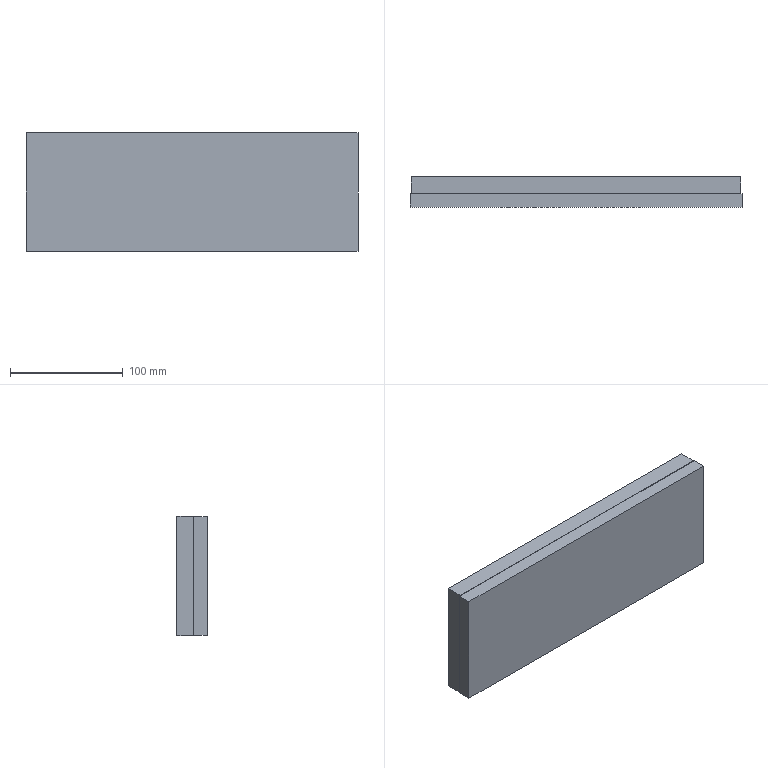NC program | NX | posted with a generic post | part box 295 x 27 x 106 mm
Lines 3310 to 4614 of 7486:
(PLANAR_MILL_6 , TOOL : D4R0)
N6474 T06 M6
N6476 G54
N6478 G17 G0 G90 X25.171 Y86.748 S3000 M3
N6480 G43 Z20. H6
N6482 Z0.3
N6484 G94 G1 X25.263 Y86.696 Z0.296 F400.
N6486 X25.737 Z0.28
N6488 X26.172 Y86.944 Z0.262
N6490 X26.42 Y87.379 Z0.245
N6492 Y87.852 Z0.228
N6494 X26.172 Y88.287 Z0.211
N6496 X25.737 Y88.536 Z0.193
N6498 X25.263 Z0.177
N6500 X24.828 Y88.287 Z0.159
N6502 X24.58 Y87.852 Z0.142
N6504 Y87.379 Z0.125
N6506 X24.828 Y86.944 Z0.108
N6508 X25.263 Y86.696 Z0.09
N6510 X25.737 Z0.074
N6512 X26.172 Y86.944 Z0.056
N6514 X26.42 Y87.379 Z0.039
N6516 Y87.852 Z0.022
N6518 X26.172 Y88.287 Z0.005
N6520 X25.737 Y88.536 Z-0.013
N6522 X25.263 Z-0.029
N6524 X24.828 Y88.287 Z-0.047
N6526 X24.58 Y87.852 Z-0.064
N6528 Y87.379 Z-0.081
N6530 X24.828 Y86.944 Z-0.098
N6532 X25.263 Y86.696 Z-0.116
N6534 X25.737 Z-0.132
N6536 X26.172 Y86.944 Z-0.15
N6538 X26.42 Y87.379 Z-0.167
N6540 Y87.852 Z-0.184
N6542 X26.172 Y88.287 Z-0.201
N6544 X25.737 Y88.536 Z-0.219
N6546 X25.263 Z-0.235
N6548 X24.828 Y88.287 Z-0.253
N6550 X24.58 Y87.852 Z-0.27
N6552 Y87.379 Z-0.287
N6554 X24.828 Y86.944 Z-0.304
N6556 X25.263 Y86.696 Z-0.322
N6558 X25.737 Z-0.338
N6560 X26.172 Y86.944 Z-0.356
N6562 X26.42 Y87.379 Z-0.373
N6564 Y87.852 Z-0.39
N6566 X26.172 Y88.287 Z-0.407
N6568 X25.737 Y88.536 Z-0.425
N6570 X25.263 Z-0.441
N6572 X24.828 Y88.287 Z-0.459
N6574 X24.58 Y87.852 Z-0.476
N6576 Y87.379 Z-0.493
N6578 X24.828 Y86.944 Z-0.51
N6580 X25.263 Y86.696 Z-0.528
N6582 X25.737 Z-0.545
N6584 X26.172 Y86.944 Z-0.562
N6586 X26.42 Y87.379 Z-0.579
N6588 Y87.852 Z-0.596
N6590 X26.172 Y88.287 Z-0.614
N6592 X25.737 Y88.536 Z-0.631
N6594 X25.263 Z-0.648
N6596 X24.828 Y88.287 Z-0.665
N6598 X24.58 Y87.852 Z-0.683
N6600 Y87.379 Z-0.699
N6602 X24.828 Y86.944 Z-0.717
N6604 X25.263 Y86.696 Z-0.734
N6606 X25.737 Z-0.751
N6608 X26.172 Y86.944 Z-0.768
N6610 X26.42 Y87.379 Z-0.786
N6612 Y87.852 Z-0.802
N6614 X26.172 Y88.287 Z-0.82
N6616 X25.737 Y88.536 Z-0.837
N6618 X25.263 Z-0.854
N6620 X24.828 Y88.287 Z-0.871
N6622 X24.58 Y87.852 Z-0.889
N6624 Y87.379 Z-0.905
N6626 X24.828 Y86.944 Z-0.923
N6628 X25.263 Y86.696 Z-0.94
N6630 X25.737 Z-0.957
N6632 X26.172 Y86.944 Z-0.974
N6634 X26.42 Y87.379 Z-0.992
N6636 Y87.852 Z-1.008
N6638 X26.172 Y88.287 Z-1.026
N6640 X25.737 Y88.536 Z-1.043
N6642 X25.263 Z-1.06
N6644 X24.828 Y88.287 Z-1.077
N6646 X24.58 Y87.852 Z-1.095
N6648 Y87.379 Z-1.111
N6650 X24.828 Y86.944 Z-1.129
N6652 X25.263 Y86.696 Z-1.146
N6654 X25.737 Z-1.163
N6656 X26.172 Y86.944 Z-1.18
N6658 X26.42 Y87.379 Z-1.198
N6660 Y87.852 Z-1.214
N6662 X26.172 Y88.287 Z-1.232
N6664 X25.737 Y88.536 Z-1.249
N6666 X25.263 Z-1.266
N6668 X24.828 Y88.287 Z-1.283
N6670 X24.58 Y87.852 Z-1.301
N6672 Y87.379 Z-1.317
N6674 X24.828 Y86.944 Z-1.335
N6676 X25.263 Y86.696 Z-1.352
N6678 X25.737 Z-1.369
N6680 X26.172 Y86.944 Z-1.386
N6682 X26.42 Y87.379 Z-1.404
N6684 Y87.852 Z-1.42
N6686 X26.172 Y88.287 Z-1.438
N6688 X25.737 Y88.536 Z-1.455
N6690 X25.263 Z-1.472
N6692 X24.828 Y88.287 Z-1.489
N6694 X24.58 Y87.852 Z-1.507
N6696 Y87.379 Z-1.523
N6698 X24.828 Y86.944 Z-1.541
N6700 X25.263 Y86.696 Z-1.558
N6702 X25.737 Z-1.575
N6704 X26.172 Y86.944 Z-1.592
N6706 X26.42 Y87.379 Z-1.61
N6708 Y87.852 Z-1.626
N6710 X26.172 Y88.287 Z-1.644
N6712 X25.737 Y88.536 Z-1.661
N6714 X25.263 Z-1.678
N6716 X24.828 Y88.287 Z-1.695
N6718 X24.58 Y87.852 Z-1.713
N6720 Y87.379 Z-1.729
N6722 X24.828 Y86.944 Z-1.747
N6724 X25.263 Y86.696 Z-1.764
N6726 X25.737 Z-1.781
N6728 X26.172 Y86.944 Z-1.798
N6730 X26.42 Y87.379 Z-1.816
N6732 Y87.852 Z-1.832
N6734 X26.172 Y88.287 Z-1.85
N6736 X25.737 Y88.536 Z-1.867
N6738 X25.263 Z-1.884
N6740 X24.828 Y88.287 Z-1.901
N6742 X24.58 Y87.852 Z-1.919
N6744 Y87.379 Z-1.935
N6746 X24.828 Y86.944 Z-1.953
N6748 X25.263 Y86.696 Z-1.97
N6750 X25.737 Z-1.987
N6752 X26.172 Y86.944 Z-2.004
N6754 X26.42 Y87.379 Z-2.022
N6756 Y87.852 Z-2.038
N6758 X26.172 Y88.287 Z-2.056
N6760 X25.737 Y88.536 Z-2.073
N6762 X25.263 Z-2.09
N6764 X24.828 Y88.287 Z-2.107
N6766 X24.58 Y87.852 Z-2.125
N6768 Y87.379 Z-2.142
N6770 X24.828 Y86.944 Z-2.159
N6772 X25.263 Y86.696 Z-2.176
N6774 X25.737 Z-2.193
N6776 X26.172 Y86.944 Z-2.211
N6778 X26.42 Y87.379 Z-2.228
N6780 Y87.852 Z-2.245
N6782 X26.172 Y88.287 Z-2.262
N6784 X25.737 Y88.536 Z-2.28
N6786 X25.263 Z-2.296
N6788 X24.828 Y88.287 Z-2.314
N6790 X24.58 Y87.852 Z-2.331
N6792 Y87.379 Z-2.348
N6794 X24.828 Y86.944 Z-2.365
N6796 X25.263 Y86.696 Z-2.383
N6798 X25.737 Z-2.399
N6800 X26.172 Y86.944 Z-2.417
N6802 X26.42 Y87.379 Z-2.434
N6804 Y87.852 Z-2.451
N6806 X26.172 Y88.287 Z-2.468
N6808 X25.737 Y88.536 Z-2.486
N6810 X25.263 Z-2.502
N6812 X24.828 Y88.287 Z-2.52
N6814 X24.58 Y87.852 Z-2.537
N6816 Y87.379 Z-2.554
N6818 X24.828 Y86.944 Z-2.571
N6820 X25.263 Y86.696 Z-2.589
N6822 X25.737 Z-2.605
N6824 X26.172 Y86.944 Z-2.623
N6826 X26.42 Y87.379 Z-2.64
N6828 Y87.852 Z-2.657
N6830 X26.172 Y88.287 Z-2.674
N6832 X25.737 Y88.536 Z-2.692
N6834 X25.263 Z-2.708
N6836 X24.828 Y88.287 Z-2.726
N6838 X24.58 Y87.852 Z-2.743
N6840 Y87.379 Z-2.76
N6842 X24.828 Y86.944 Z-2.777
N6844 X25.263 Y86.696 Z-2.795
N6846 X25.737 Z-2.811
N6848 X26.172 Y86.944 Z-2.829
N6850 X26.42 Y87.379 Z-2.846
N6852 Y87.852 Z-2.863
N6854 X26.172 Y88.287 Z-2.88
N6856 X25.737 Y88.536 Z-2.898
N6858 X25.263 Z-2.914
N6860 X24.828 Y88.287 Z-2.932
N6862 X24.58 Y87.852 Z-2.949
N6864 Y87.379 Z-2.966
N6866 X24.828 Y86.944 Z-2.983
N6868 X25.263 Y86.696 Z-3.001
N6870 X25.737 Z-3.017
N6872 X26.172 Y86.944 Z-3.035
N6874 X26.42 Y87.379 Z-3.052
N6876 Y87.852 Z-3.069
N6878 X26.172 Y88.287 Z-3.086
N6880 X25.737 Y88.536 Z-3.104
N6882 X25.263 Z-3.12
N6884 X24.828 Y88.287 Z-3.138
N6886 X24.58 Y87.852 Z-3.155
N6888 Y87.379 Z-3.172
N6890 X24.828 Y86.944 Z-3.189
N6892 X25.263 Y86.696 Z-3.207
N6894 X25.737 Z-3.223
N6896 X26.172 Y86.944 Z-3.241
N6898 X26.42 Y87.379 Z-3.258
N6900 Y87.852 Z-3.275
N6902 X26.172 Y88.287 Z-3.292
N6904 X25.737 Y88.536 Z-3.31
N6906 X25.263 Z-3.326
N6908 X24.828 Y88.287 Z-3.344
N6910 X24.58 Y87.852 Z-3.361
N6912 Y87.379 Z-3.378
N6914 X24.828 Y86.944 Z-3.395
N6916 X25.263 Y86.696 Z-3.413
N6918 X25.737 Z-3.429
N6920 X26.172 Y86.944 Z-3.447
N6922 X26.42 Y87.379 Z-3.464
N6924 Y87.852 Z-3.481
N6926 X26.172 Y88.287 Z-3.498
N6928 X25.737 Y88.536 Z-3.516
N6930 X25.263 Z-3.532
N6932 X24.828 Y88.287 Z-3.55
N6934 X24.58 Y87.852 Z-3.567
N6936 Y87.379 Z-3.584
N6938 X24.828 Y86.944 Z-3.601
N6940 X25.263 Y86.696 Z-3.619
N6942 X25.737 Z-3.635
N6944 X26.172 Y86.944 Z-3.653
N6946 X26.42 Y87.379 Z-3.67
N6948 Y87.852 Z-3.687
N6950 X26.172 Y88.287 Z-3.704
N6952 X25.737 Y88.536 Z-3.722
N6954 X25.263 Z-3.739
N6956 X24.828 Y88.287 Z-3.756
N6958 X24.58 Y87.852 Z-3.773
N6960 Y87.379 Z-3.79
N6962 X24.828 Y86.944 Z-3.808
N6964 X25.263 Y86.696 Z-3.825
N6966 X25.737 Z-3.842
N6968 X26.172 Y86.944 Z-3.859
N6970 X26.42 Y87.379 Z-3.877
N6972 Y87.852 Z-3.893
N6974 X26.172 Y88.287 Z-3.911
N6976 X25.737 Y88.536 Z-3.928
N6978 X25.263 Z-3.945
N6980 X24.828 Y88.287 Z-3.962
N6982 X24.58 Y87.852 Z-3.98
N6984 Y87.379 Z-3.996
N6986 X24.828 Y86.944 Z-4.014
N6988 X25.263 Y86.696 Z-4.031
N6990 X25.737 Z-4.048
N6992 X26.172 Y86.944 Z-4.065
N6994 X26.42 Y87.379 Z-4.083
N6996 Y87.852 Z-4.099
N6998 X26.172 Y88.287 Z-4.117
N7000 X25.737 Y88.536 Z-4.134
N7002 X25.263 Z-4.151
N7004 X24.828 Y88.287 Z-4.168
N7006 X24.58 Y87.852 Z-4.186
N7008 Y87.379 Z-4.202
N7010 X24.828 Y86.944 Z-4.22
N7012 X25.263 Y86.696 Z-4.237
N7014 X25.737 Z-4.254
N7016 X26.172 Y86.944 Z-4.271
N7018 X26.42 Y87.379 Z-4.289
N7020 Y87.852 Z-4.305
N7022 X26.172 Y88.287 Z-4.323
N7024 X25.737 Y88.536 Z-4.34
N7026 X25.263 Z-4.357
N7028 X24.828 Y88.287 Z-4.374
N7030 X24.58 Y87.852 Z-4.392
N7032 Y87.379 Z-4.408
N7034 X24.828 Y86.944 Z-4.426
N7036 X25.263 Y86.696 Z-4.443
N7038 X25.737 Z-4.46
N7040 X26.172 Y86.944 Z-4.477
N7042 X26.42 Y87.379 Z-4.495
N7044 Y87.852 Z-4.511
N7046 X26.172 Y88.287 Z-4.529
N7048 X25.737 Y88.536 Z-4.546
N7050 X25.263 Z-4.563
N7052 X24.828 Y88.287 Z-4.58
N7054 X24.58 Y87.852 Z-4.598
N7056 Y87.379 Z-4.614
N7058 X24.828 Y86.944 Z-4.632
N7060 X25.263 Y86.696 Z-4.649
N7062 X25.737 Z-4.666
N7064 X26.172 Y86.944 Z-4.683
N7066 X26.42 Y87.379 Z-4.701
N7068 Y87.852 Z-4.717
N7070 X26.172 Y88.287 Z-4.735
N7072 X25.737 Y88.536 Z-4.752
N7074 X25.263 Z-4.769
N7076 X24.828 Y88.287 Z-4.786
N7078 X24.58 Y87.852 Z-4.804
N7080 Y87.379 Z-4.82
N7082 X24.828 Y86.944 Z-4.838
N7084 X25.263 Y86.696 Z-4.855
N7086 X25.737 Z-4.872
N7088 X26.172 Y86.944 Z-4.889
N7090 X26.42 Y87.379 Z-4.907
N7092 Y87.852 Z-4.923
N7094 X26.172 Y88.287 Z-4.941
N7096 X25.737 Y88.536 Z-4.958
N7098 X25.263 Z-4.975
N7100 X24.828 Y88.287 Z-4.992
N7102 X24.58 Y87.852 Z-5.01
N7104 Y87.379 Z-5.026
N7106 X24.828 Y86.944 Z-5.044
N7108 X25.263 Y86.696 Z-5.061
N7110 X25.737 Z-5.078
N7112 X26.172 Y86.944 Z-5.095
N7114 X26.42 Y87.379 Z-5.113
N7116 Y87.852 Z-5.129
N7118 X26.172 Y88.287 Z-5.147
N7120 X25.737 Y88.536 Z-5.164
N7122 X25.263 Z-5.181
N7124 X24.828 Y88.287 Z-5.198
N7126 X24.58 Y87.852 Z-5.216
N7128 Y87.379 Z-5.232
N7130 X24.828 Y86.944 Z-5.25
N7132 X25.263 Y86.696 Z-5.267
N7134 X25.737 Z-5.284
N7136 X26.172 Y86.944 Z-5.301
N7138 X26.42 Y87.379 Z-5.319
N7140 Y87.852 Z-5.336
N7142 X26.172 Y88.287 Z-5.353
N7144 X25.737 Y88.536 Z-5.371
N7146 X25.263 Z-5.387
N7148 X24.828 Y88.287 Z-5.405
N7150 X24.58 Y87.852 Z-5.422
N7152 Y87.379 Z-5.439
N7154 X24.828 Y86.944 Z-5.456
N7156 X25.263 Y86.696 Z-5.474
N7158 X25.737 Z-5.49
N7160 X26.172 Y86.944 Z-5.508
N7162 X26.42 Y87.379 Z-5.525
N7164 Y87.852 Z-5.542
N7166 X26.172 Y88.287 Z-5.559
N7168 X25.737 Y88.536 Z-5.577
N7170 X25.263 Z-5.593
N7172 X24.828 Y88.287 Z-5.611
N7174 X24.58 Y87.852 Z-5.628
N7176 Y87.379 Z-5.645
N7178 X24.828 Y86.944 Z-5.662
N7180 X25.263 Y86.696 Z-5.68
N7182 X25.737 Z-5.696
N7184 X26.172 Y86.944 Z-5.714
N7186 X26.42 Y87.379 Z-5.731
N7188 Y87.852 Z-5.748
N7190 X26.172 Y88.287 Z-5.765
N7192 X25.737 Y88.536 Z-5.783
N7194 X25.263 Z-5.799
N7196 X24.828 Y88.287 Z-5.817
N7198 X24.58 Y87.852 Z-5.834
N7200 Y87.379 Z-5.851
N7202 X24.828 Y86.944 Z-5.868
N7204 X25.263 Y86.696 Z-5.886
N7206 X25.737 Z-5.902
N7208 X26.172 Y86.944 Z-5.92
N7210 X26.42 Y87.379 Z-5.937
N7212 Y87.852 Z-5.954
N7214 X26.172 Y88.287 Z-5.971
N7216 X25.737 Y88.536 Z-5.989
N7218 X25.263 Z-6.005
N7220 X24.828 Y88.287 Z-6.023
N7222 X24.58 Y87.852 Z-6.04
N7224 Y87.379 Z-6.057
N7226 X24.828 Y86.944 Z-6.074
N7228 X25.263 Y86.696 Z-6.092
N7230 X25.5 Z-6.1
N7232 G3 X26.42 Y87.616 R0.92
N7234 X25.5 Y86.696 R-0.92
N7236 G1 Z-5.8
N7238 G0 Z20.
N7240 X244.171 Y48.133
N7242 Z0.3
N7244 G1 X244.263 Y48.08 Z0.296
N7246 X244.737 Z0.28
N7248 X245.172 Y48.328 Z0.262
N7250 X245.42 Y48.763 Z0.245
N7252 Y49.237 Z0.228
N7254 X245.172 Y49.672 Z0.211
N7256 X244.737 Y49.92 Z0.193
N7258 X244.263 Z0.177
N7260 X243.828 Y49.672 Z0.159
N7262 X243.58 Y49.237 Z0.142
N7264 Y48.763 Z0.125
N7266 X243.828 Y48.328 Z0.108
N7268 X244.263 Y48.08 Z0.09
N7270 X244.737 Z0.074
N7272 X245.172 Y48.328 Z0.056
N7274 X245.42 Y48.763 Z0.039
N7276 Y49.237 Z0.022
N7278 X245.172 Y49.672 Z0.005
N7280 X244.737 Y49.92 Z-0.013
N7282 X244.263 Z-0.029
N7284 X243.828 Y49.672 Z-0.047
N7286 X243.58 Y49.237 Z-0.064
N7288 Y48.763 Z-0.081
N7290 X243.828 Y48.328 Z-0.098
N7292 X244.263 Y48.08 Z-0.116
N7294 X244.737 Z-0.132
N7296 X245.172 Y48.328 Z-0.15
N7298 X245.42 Y48.763 Z-0.167
N7300 Y49.237 Z-0.184
N7302 X245.172 Y49.672 Z-0.201
N7304 X244.737 Y49.92 Z-0.219
N7306 X244.263 Z-0.235
N7308 X243.828 Y49.672 Z-0.253
N7310 X243.58 Y49.237 Z-0.27
N7312 Y48.763 Z-0.287
N7314 X243.828 Y48.328 Z-0.304
N7316 X244.263 Y48.08 Z-0.322
N7318 X244.737 Z-0.338
N7320 X245.172 Y48.328 Z-0.356
N7322 X245.42 Y48.763 Z-0.373
N7324 Y49.237 Z-0.39
N7326 X245.172 Y49.672 Z-0.407
N7328 X244.737 Y49.92 Z-0.425
N7330 X244.263 Z-0.441
N7332 X243.828 Y49.672 Z-0.459
N7334 X243.58 Y49.237 Z-0.476
N7336 Y48.763 Z-0.493
N7338 X243.828 Y48.328 Z-0.51
N7340 X244.263 Y48.08 Z-0.528
N7342 X244.737 Z-0.545
N7344 X245.172 Y48.328 Z-0.562
N7346 X245.42 Y48.763 Z-0.579
N7348 Y49.237 Z-0.596
N7350 X245.172 Y49.672 Z-0.614
N7352 X244.737 Y49.92 Z-0.631
N7354 X244.263 Z-0.648
N7356 X243.828 Y49.672 Z-0.665
N7358 X243.58 Y49.237 Z-0.683
N7360 Y48.763 Z-0.699
N7362 X243.828 Y48.328 Z-0.717
N7364 X244.263 Y48.08 Z-0.734
N7366 X244.737 Z-0.751
N7368 X245.172 Y48.328 Z-0.768
N7370 X245.42 Y48.763 Z-0.786
N7372 Y49.237 Z-0.802
N7374 X245.172 Y49.672 Z-0.82
N7376 X244.737 Y49.92 Z-0.837
N7378 X244.263 Z-0.854
N7380 X243.828 Y49.672 Z-0.871
N7382 X243.58 Y49.237 Z-0.889
N7384 Y48.763 Z-0.905
N7386 X243.828 Y48.328 Z-0.923
N7388 X244.263 Y48.08 Z-0.94
N7390 X244.737 Z-0.957
N7392 X245.172 Y48.328 Z-0.974
N7394 X245.42 Y48.763 Z-0.992
N7396 Y49.237 Z-1.008
N7398 X245.172 Y49.672 Z-1.026
N7400 X244.737 Y49.92 Z-1.043
N7402 X244.263 Z-1.06
N7404 X243.828 Y49.672 Z-1.077
N7406 X243.58 Y49.237 Z-1.095
N7408 Y48.763 Z-1.111
N7410 X243.828 Y48.328 Z-1.129
N7412 X244.263 Y48.08 Z-1.146
N7414 X244.737 Z-1.163
N7416 X245.172 Y48.328 Z-1.18
N7418 X245.42 Y48.763 Z-1.198
N7420 Y49.237 Z-1.214
N7422 X245.172 Y49.672 Z-1.232
N7424 X244.737 Y49.92 Z-1.249
N7426 X244.263 Z-1.266
N7428 X243.828 Y49.672 Z-1.283
N7430 X243.58 Y49.237 Z-1.301
N7432 Y48.763 Z-1.317
N7434 X243.828 Y48.328 Z-1.335
N7436 X244.263 Y48.08 Z-1.352
N7438 X244.737 Z-1.369
N7440 X245.172 Y48.328 Z-1.386
N7442 X245.42 Y48.763 Z-1.404
N7444 Y49.237 Z-1.42
N7446 X245.172 Y49.672 Z-1.438
N7448 X244.737 Y49.92 Z-1.455
N7450 X244.263 Z-1.472
N7452 X243.828 Y49.672 Z-1.489
N7454 X243.58 Y49.237 Z-1.507
N7456 Y48.763 Z-1.523
N7458 X243.828 Y48.328 Z-1.541
N7460 X244.263 Y48.08 Z-1.558
N7462 X244.737 Z-1.575
N7464 X245.172 Y48.328 Z-1.592
N7466 X245.42 Y48.763 Z-1.61
N7468 Y49.237 Z-1.626
N7470 X245.172 Y49.672 Z-1.644
N7472 X244.737 Y49.92 Z-1.661
N7474 X244.263 Z-1.678
N7476 X243.828 Y49.672 Z-1.695
N7478 X243.58 Y49.237 Z-1.713
N7480 Y48.763 Z-1.729
N7482 X243.828 Y48.328 Z-1.747
N7484 X244.263 Y48.08 Z-1.764
N7486 X244.737 Z-1.781
N7488 X245.172 Y48.328 Z-1.798
N7490 X245.42 Y48.763 Z-1.816
N7492 Y49.237 Z-1.832
N7494 X245.172 Y49.672 Z-1.85
N7496 X244.737 Y49.92 Z-1.867
N7498 X244.263 Z-1.884
N7500 X243.828 Y49.672 Z-1.901
N7502 X243.58 Y49.237 Z-1.919
N7504 Y48.763 Z-1.935
N7506 X243.828 Y48.328 Z-1.953
N7508 X244.263 Y48.08 Z-1.97
N7510 X244.737 Z-1.987
N7512 X245.172 Y48.328 Z-2.004
N7514 X245.42 Y48.763 Z-2.022
N7516 Y49.237 Z-2.038
N7518 X245.172 Y49.672 Z-2.056
N7520 X244.737 Y49.92 Z-2.073
N7522 X244.263 Z-2.09
N7524 X243.828 Y49.672 Z-2.107
N7526 X243.58 Y49.237 Z-2.125
N7528 Y48.763 Z-2.142
N7530 X243.828 Y48.328 Z-2.159
N7532 X244.263 Y48.08 Z-2.176
N7534 X244.737 Z-2.193
N7536 X245.172 Y48.328 Z-2.211
N7538 X245.42 Y48.763 Z-2.228
N7540 Y49.237 Z-2.245
N7542 X245.172 Y49.672 Z-2.262
N7544 X244.737 Y49.92 Z-2.28
N7546 X244.263 Z-2.296
N7548 X243.828 Y49.672 Z-2.314
N7550 X243.58 Y49.237 Z-2.331
N7552 Y48.763 Z-2.348
N7554 X243.828 Y48.328 Z-2.365
N7556 X244.263 Y48.08 Z-2.383
N7558 X244.737 Z-2.399
N7560 X245.172 Y48.328 Z-2.417
N7562 X245.42 Y48.763 Z-2.434
N7564 Y49.237 Z-2.451
N7566 X245.172 Y49.672 Z-2.468
N7568 X244.737 Y49.92 Z-2.486
N7570 X244.263 Z-2.502
N7572 X243.828 Y49.672 Z-2.52
N7574 X243.58 Y49.237 Z-2.537
N7576 Y48.763 Z-2.554
N7578 X243.828 Y48.328 Z-2.571
N7580 X244.263 Y48.08 Z-2.589
N7582 X244.737 Z-2.605
N7584 X245.172 Y48.328 Z-2.623
N7586 X245.42 Y48.763 Z-2.64
N7588 Y49.237 Z-2.657
N7590 X245.172 Y49.672 Z-2.674
N7592 X244.737 Y49.92 Z-2.692
N7594 X244.263 Z-2.708
N7596 X243.828 Y49.672 Z-2.726
N7598 X243.58 Y49.237 Z-2.743
N7600 Y48.763 Z-2.76
N7602 X243.828 Y48.328 Z-2.777
N7604 X244.263 Y48.08 Z-2.795
N7606 X244.737 Z-2.811
N7608 X245.172 Y48.328 Z-2.829
N7610 X245.42 Y48.763 Z-2.846
N7612 Y49.237 Z-2.863
N7614 X245.172 Y49.672 Z-2.88
N7616 X244.737 Y49.92 Z-2.898
N7618 X244.263 Z-2.914
N7620 X243.828 Y49.672 Z-2.932
N7622 X243.58 Y49.237 Z-2.949
N7624 Y48.763 Z-2.966
N7626 X243.828 Y48.328 Z-2.983
N7628 X244.263 Y48.08 Z-3.001
N7630 X244.737 Z-3.017
N7632 X245.172 Y48.328 Z-3.035
N7634 X245.42 Y48.763 Z-3.052
N7636 Y49.237 Z-3.069
N7638 X245.172 Y49.672 Z-3.086
N7640 X244.737 Y49.92 Z-3.104
N7642 X244.263 Z-3.12
N7644 X243.828 Y49.672 Z-3.138
N7646 X243.58 Y49.237 Z-3.155
N7648 Y48.763 Z-3.172
N7650 X243.828 Y48.328 Z-3.189
N7652 X244.263 Y48.08 Z-3.207
N7654 X244.737 Z-3.223
N7656 X245.172 Y48.328 Z-3.241
N7658 X245.42 Y48.763 Z-3.258
N7660 Y49.237 Z-3.275
N7662 X245.172 Y49.672 Z-3.292
N7664 X244.737 Y49.92 Z-3.31
N7666 X244.263 Z-3.326
N7668 X243.828 Y49.672 Z-3.344
N7670 X243.58 Y49.237 Z-3.361
N7672 Y48.763 Z-3.378
N7674 X243.828 Y48.328 Z-3.395
N7676 X244.263 Y48.08 Z-3.413
N7678 X244.737 Z-3.429
N7680 X245.172 Y48.328 Z-3.447
N7682 X245.42 Y48.763 Z-3.464
N7684 Y49.237 Z-3.481
N7686 X245.172 Y49.672 Z-3.498
N7688 X244.737 Y49.92 Z-3.516
N7690 X244.263 Z-3.532
N7692 X243.828 Y49.672 Z-3.55
N7694 X243.58 Y49.237 Z-3.567
N7696 Y48.763 Z-3.584
N7698 X243.828 Y48.328 Z-3.601
N7700 X244.263 Y48.08 Z-3.619
N7702 X244.737 Z-3.635
N7704 X245.172 Y48.328 Z-3.653
N7706 X245.42 Y48.763 Z-3.67
N7708 Y49.237 Z-3.687
N7710 X245.172 Y49.672 Z-3.704
N7712 X244.737 Y49.92 Z-3.722
N7714 X244.263 Z-3.739
N7716 X243.828 Y49.672 Z-3.756
N7718 X243.58 Y49.237 Z-3.773
N7720 Y48.763 Z-3.79
N7722 X243.828 Y48.328 Z-3.808
N7724 X244.263 Y48.08 Z-3.825
N7726 X244.737 Z-3.842
N7728 X245.172 Y48.328 Z-3.859
N7730 X245.42 Y48.763 Z-3.877
N7732 Y49.237 Z-3.893
N7734 X245.172 Y49.672 Z-3.911
N7736 X244.737 Y49.92 Z-3.928
N7738 X244.263 Z-3.945
N7740 X243.828 Y49.672 Z-3.962
N7742 X243.58 Y49.237 Z-3.98
N7744 Y48.763 Z-3.996
N7746 X243.828 Y48.328 Z-4.014
N7748 X244.263 Y48.08 Z-4.031
N7750 X244.737 Z-4.048
N7752 X245.172 Y48.328 Z-4.065
N7754 X245.42 Y48.763 Z-4.083
N7756 Y49.237 Z-4.099
N7758 X245.172 Y49.672 Z-4.117
N7760 X244.737 Y49.92 Z-4.134
N7762 X244.263 Z-4.151
N7764 X243.828 Y49.672 Z-4.168
N7766 X243.58 Y49.237 Z-4.186
N7768 Y48.763 Z-4.202
N7770 X243.828 Y48.328 Z-4.22
N7772 X244.263 Y48.08 Z-4.237
N7774 X244.737 Z-4.254
N7776 X245.172 Y48.328 Z-4.271
N7778 X245.42 Y48.763 Z-4.289
N7780 Y49.237 Z-4.305
N7782 X245.172 Y49.672 Z-4.323
N7784 X244.737 Y49.92 Z-4.34
N7786 X244.263 Z-4.357
N7788 X243.828 Y49.672 Z-4.374
N7790 X243.58 Y49.237 Z-4.392
N7792 Y48.763 Z-4.408
N7794 X243.828 Y48.328 Z-4.426
N7796 X244.263 Y48.08 Z-4.443
N7798 X244.737 Z-4.46
N7800 X245.172 Y48.328 Z-4.477
N7802 X245.42 Y48.763 Z-4.495
N7804 Y49.237 Z-4.511
N7806 X245.172 Y49.672 Z-4.529
N7808 X244.737 Y49.92 Z-4.546
N7810 X244.263 Z-4.563
N7812 X243.828 Y49.672 Z-4.58
N7814 X243.58 Y49.237 Z-4.598
N7816 Y48.763 Z-4.614
N7818 X243.828 Y48.328 Z-4.632
N7820 X244.263 Y48.08 Z-4.649
N7822 X244.737 Z-4.666
N7824 X245.172 Y48.328 Z-4.683
N7826 X245.42 Y48.763 Z-4.701
N7828 Y49.237 Z-4.717
N7830 X245.172 Y49.672 Z-4.735
N7832 X244.737 Y49.92 Z-4.752
N7834 X244.263 Z-4.769
N7836 X243.828 Y49.672 Z-4.786
N7838 X243.58 Y49.237 Z-4.804
N7840 Y48.763 Z-4.82
N7842 X243.828 Y48.328 Z-4.838
N7844 X244.263 Y48.08 Z-4.855
N7846 X244.737 Z-4.872
N7848 X245.172 Y48.328 Z-4.889
N7850 X245.42 Y48.763 Z-4.907
N7852 Y49.237 Z-4.923
N7854 X245.172 Y49.672 Z-4.941
N7856 X244.737 Y49.92 Z-4.958
N7858 X244.263 Z-4.975
N7860 X243.828 Y49.672 Z-4.992
N7862 X243.58 Y49.237 Z-5.01
N7864 Y48.763 Z-5.026
N7866 X243.828 Y48.328 Z-5.044
N7868 X244.263 Y48.08 Z-5.061
N7870 X244.737 Z-5.078
N7872 X245.172 Y48.328 Z-5.095
N7874 X245.42 Y48.763 Z-5.113
N7876 Y49.237 Z-5.129
N7878 X245.172 Y49.672 Z-5.147
N7880 X244.737 Y49.92 Z-5.164
N7882 X244.263 Z-5.181
N7884 X243.828 Y49.672 Z-5.198
N7886 X243.58 Y49.237 Z-5.216
N7888 Y48.763 Z-5.232
N7890 X243.828 Y48.328 Z-5.25
N7892 X244.263 Y48.08 Z-5.267
N7894 X244.737 Z-5.284
N7896 X245.172 Y48.328 Z-5.301
N7898 X245.42 Y48.763 Z-5.319
N7900 Y49.237 Z-5.336
N7902 X245.172 Y49.672 Z-5.353
N7904 X244.737 Y49.92 Z-5.371
N7906 X244.263 Z-5.387
N7908 X243.828 Y49.672 Z-5.405
N7910 X243.58 Y49.237 Z-5.422
N7912 Y48.763 Z-5.439
N7914 X243.828 Y48.328 Z-5.456
N7916 X244.263 Y48.08 Z-5.474
N7918 X244.737 Z-5.49
N7920 X245.172 Y48.328 Z-5.508
N7922 X245.42 Y48.763 Z-5.525
N7924 Y49.237 Z-5.542
N7926 X245.172 Y49.672 Z-5.559
N7928 X244.737 Y49.92 Z-5.577
N7930 X244.263 Z-5.593
N7932 X243.828 Y49.672 Z-5.611
N7934 X243.58 Y49.237 Z-5.628
N7936 Y48.763 Z-5.645
N7938 X243.828 Y48.328 Z-5.662
N7940 X244.263 Y48.08 Z-5.68
N7942 X244.737 Z-5.696
N7944 X245.172 Y48.328 Z-5.714
N7946 X245.42 Y48.763 Z-5.731
N7948 Y49.237 Z-5.748
N7950 X245.172 Y49.672 Z-5.765
N7952 X244.737 Y49.92 Z-5.783
N7954 X244.263 Z-5.799
N7956 X243.828 Y49.672 Z-5.817
N7958 X243.58 Y49.237 Z-5.834
N7960 Y48.763 Z-5.851
N7962 X243.828 Y48.328 Z-5.868
N7964 X244.263 Y48.08 Z-5.886
N7966 X244.737 Z-5.902
N7968 X245.172 Y48.328 Z-5.92
N7970 X245.42 Y48.763 Z-5.937
N7972 Y49.237 Z-5.954
N7974 X245.172 Y49.672 Z-5.971
N7976 X244.737 Y49.92 Z-5.989
N7978 X244.263 Z-6.005
N7980 X243.828 Y49.672 Z-6.023
N7982 X243.58 Y49.237 Z-6.04
N7984 Y48.763 Z-6.057
N7986 X243.828 Y48.328 Z-6.074
N7988 X244.263 Y48.08 Z-6.092
N7990 X244.5 Z-6.1
N7992 G3 X245.42 Y49. R0.92
N7994 X244.5 Y48.08 R-0.92
N7996 G1 Z-5.8
N7998 G0 Z20.
(PLANAR_MILL_6_COPY , TOOL : D4R0)
N8000 X25.335 Y87.069
N8002 Z-3.05
N8004 G1 Z-6.05 F150.
N8006 G41 X25.3 Y86.872 D6
N8008 Y86.846
N8010 G3 X25.5 Y86.646 R0.2
N8012 X26.47 Y87.616 R0.97
N8014 X25.5 Y86.646 R-0.97
N8016 X25.7 Y86.846 R0.2
N8018 G40
N8020 G1 X25.665 Y87.043
N8022 X25.335
N8024 G41 X25.3 Y86.846
N8026 G3 X25.5 Y86.646 R0.2
N8028 X26.47 Y87.616 R0.97
N8030 X25.5 Y86.646 R-0.97
N8032 X25.7 Y86.846 R0.2
N8034 G1 Y86.872
N8036 G40
N8038 X25.665 Y87.069
N8040 Z-3.05
N8042 G0 Z20.
N8044 X244.335 Y48.453
N8046 Z-3.05
N8048 G1 Z-6.05
N8050 G41 X244.3 Y48.256
N8052 Y48.23
N8054 G3 X244.5 Y48.03 R0.2
N8056 X245.47 Y49. R0.97
N8058 X244.5 Y48.03 R-0.97
N8060 X244.7 Y48.23 R0.2
N8062 G40
N8064 G1 X244.665 Y48.427
N8066 X244.335
N8068 G41 X244.3 Y48.23
N8070 G3 X244.5 Y48.03 R0.2
N8072 X245.47 Y49. R0.97
N8074 X244.5 Y48.03 R-0.97
N8076 X244.7 Y48.23 R0.2
N8078 G1 Y48.256
N8080 G40
N8082 X244.665 Y48.453
N8084 Z-3.05
N8086 G0 Z20.
N8088 M5
(PLANAR_MILL_7 , TOOL : DJ-D3倒角)
N8090 T07 M6
N8092 G54
N8094 G17 G0 G90 X4.533 Y30.734 S6000 M3
N8096 G43 Z20. H7
N8098 Z2.
N8100 G94 G1 Z-1. F1000.
N8102 G3 X3.742 Y29.562 R1.
N8104 G1 X3.909 Y28.703
N8106 G3 X6.604 Y26.883 R2.3
N8108 X8.424 Y29.579 R2.3
N8110 G1 X8.091 Y31.297
N8112 G3 X5.396 Y33.117 R2.3
N8114 X3.576 Y30.421 R2.3
N8116 G1 X3.742 Y29.562
N8118 G3 X4.914 Y28.771 R1.
N8120 G1 Z2.
N8122 G0 Z20.
N8124 Y69.229
N8126 Z2.
N8128 G1 Z-1.
N8130 G3 X3.742 Y68.438 R1.
N8132 G1 X3.576 Y67.579
N8134 G3 X5.396 Y64.883 R2.3
N8136 X8.091 Y66.703 R2.3
N8138 G1 X8.424 Y68.421
N8140 G3 X6.604 Y71.117 R2.3
N8142 X3.909 Y69.297 R2.3
N8144 G1 X3.742 Y68.438
N8146 G3 X4.533 Y67.266 R1.
N8148 G1 Z2.
N8150 G0 Z20.
N8152 X26.5 Y88.616
N8154 Z2.
N8156 G1 Z-1.
N8158 G3 X25.5 Y89.616 R1.
N8160 X23.5 Y87.616 R2.
N8162 X25.5 Y89.616 R-2.
N8164 X24.5 Y88.616 R1.
N8166 G1 Z2.
N8168 G0 Z20.
N8170 X243.5 Y48.
N8172 Z2.
N8174 G1 Z-1.
N8176 G3 X244.5 Y47. R1.
N8178 X246.5 Y49. R2.
N8180 X244.5 Y47. R-2.
N8182 X245.5 Y48. R1.
N8184 G1 Z2.
N8186 G0 Z20.
N8188 X265.409 Y67.16
N8190 Z2.
N8192 G1 Z-1.
N8194 G3 X266.284 Y68.271 R1.
N8196 G1 X266.119 Y69.661
N8198 G3 X263.564 Y71.674 R2.3
N8200 X261.551 Y69.119 R2.3
N8202 G1 X261.881 Y66.339
N8204 G3 X264.436 Y64.326 R2.3
N8206 X266.449 Y66.881 R2.3
N8208 G1 X266.284 Y68.271
N8210 G3 X265.173 Y69.146 R1.
N8212 G1 Z2.
N8214 G0 Z20.
N8216 Y28.854
N8218 Z2.
N8220 G1 Z-1.
N8222 G3 X266.284 Y29.729 R1.
N8224 G1 X266.449 Y31.119
N8226 G3 X264.436 Y33.674 R2.3
N8228 X261.881 Y31.661 R2.3
N8230 G1 X261.551 Y28.881
N8232 G3 X263.564 Y26.326 R2.3
N8234 X266.119 Y28.339 R2.3
N8236 G1 X266.284 Y29.729
N8238 G3 X265.409 Y30.84 R1.
N8240 G1 Z2.
N8242 G0 Z20.
(PLANAR_MILL_7_COPY , TOOL : DJ-D3倒角)
N8244 X228.6 Y48.
N8246 Z2.6
N8248 G1 Z-0.4
N8250 G3 X229.6 Y49. R1.
N8252 G1 Y98.
N8254 G2 X230. Y98.4 R0.4
N8256 G1 X245.
N8258 G2 X254.907 Y91.164 R10.4
N8260 G3 X262.107 Y84.684 R9.6
N8262 G2 X270.4 Y74.5 R10.4
N8264 G1 Y55.5
N8266 G3 X272. Y53.9 R1.6
N8268 G1 X284.
N8270 G2 X284.283 Y53.783 R0.4
N8272 G1 X285.283 Y52.783
N8274 G2 X285.4 Y52.5 R0.4
N8276 G1 Y45.5
N8278 G2 X285.283 Y45.217 R0.4
N8280 G1 X284.283 Y44.217
N8282 G2 X284. Y44.1 R0.4
N8284 G1 X272.
N8286 G3 X270.4 Y42.5 R1.6
N8288 G1 Y23.5
N8290 G2 X262.107 Y13.316 R10.4
N8292 G3 X254.907 Y6.836 R9.6
N8294 G2 X245. Y-0.4 R10.4
N8296 G1 X230.
N8298 G2 X229.6 Y0. R0.4
N8300 G1 Y49.
N8302 G3 X228.6 Y50. R1.
N8304 G1 Z2.6
N8306 G0 Z20.
N8308 X41.4
N8310 Z2.6
N8312 G1 Z-0.4
N8314 G3 X40.4 Y49. R1.
N8316 G1 Y0.
N8318 G2 X40. Y-0.4 R0.4
N8320 G1 X25.
N8322 G2 X15.798 Y5.155 R10.4
N8324 G3 X8.598 Y10.195 R9.6
N8326 G2 X-0.4 Y20.5 R10.4
N8328 G1 Y77.5
N8330 G2 X8.598 Y87.805 R10.4
N8332 G3 X15.798 Y92.845 R9.6
N8334 G2 X25. Y98.4 R10.4
N8336 G1 X40.
N8338 G2 X40.4 Y98. R0.4
N8340 G1 Y49.
N8342 G3 X41.4 Y48. R1.
N8344 G1 Z2.6
N8346 G0 Z20.
(PLANAR_MILL_7_COPY_COPY , TOOL : DJ-D3倒角)
N8348 X105. Y91.
N8350 Z1.5
N8352 G1 Z-1.5
N8354 G3 X104. Y92. R1.
N8356 X64. Y52. R40.
N8358 X104. Y92. R-40.
N8360 X103. Y91. R1.
N8362 G1 Z1.5
N8364 G0 Z20.
(PLANAR_MILL_7_COPY_COPY_COPY , TOOL : DJ-D3倒角)
N8366 X229. Y-2.
N8368 Z1.5
N8370 G1 Z-1.5
N8372 G3 X228. Y-1. R1.
N8374 G1 X42.
N8376 G3 X41. Y-2. R1.
N8378 G1 Z1.5
N8380 G0 Z20.
N8382 Y100.
N8384 Z1.5
N8386 G1 Z-1.5
N8388 G3 X42. Y99. R1.
N8390 G1 X228.
N8392 G3 X229. Y100. R1.
N8394 G1 Z1.5
N8396 G0 Z20.
N8398 M5
(FLOOR_WALL_6_COPY , TOOL : D8R0精铣)
N8400 T03 M6
N8402 G54
N8404 G17 G0 G90 X-38.5 Y56. S3500 M3
N8406 G43 Z20. H3
N8408 Z-1.
N8410 G94 G1 Z-4. F800.
N8412 Y51.4
N8414 X-3.338
N8416 G2 X-2.7 Y50.762 R0.64
N8418 G1 Y42.843
N8420 X-1.3 Y41.591
N8422 G2 X-1.3 Y-41.591 R55.8
N8424 G1 X-2.7 Y-42.843
N8426 Y-50.762
N8428 G2 X-3.338 Y-51.4 R0.64
N8430 G1 X-73.662
N8432 G2 X-74.3 Y-50.762 R0.64
N8434 G1 Y-42.843
N8436 X-75.7 Y-41.591
N8438 G2 X-75.7 Y41.591 R55.8
N8440 G1 X-74.3 Y42.843
N8442 Y50.762
N8444 G2 X-73.662 Y51.4 R0.64
N8446 G1 X-36.842
N8448 G2 X-36.31 Y51.115 R0.64
N8450 G1 X-32.69 Y45.685
N8452 G3 X-32.158 Y45.4 R0.64
N8454 G1 X-9.337
N8456 G2 X-8.7 Y44.763 R0.64
N8458 G1 Y42.843
N8460 G3 X-6.7 Y38.371 R6.
N8462 G1 X-5.3 Y37.119
N8464 G2 X-1.381 Y-33.2 R49.8
N8466 X-5.3 Y-37.119 R49.8
N8468 G1 X-6.7 Y-38.371
N8470 G3 X-8.7 Y-42.843 R6.
N8472 G1 Y-44.763
N8474 G2 X-9.337 Y-45.4 R0.64
N8476 G1 X-67.663
N8478 G2 X-68.3 Y-44.763 R0.64
N8480 G1 Y-42.843
N8482 G3 X-70.3 Y-38.371 R6.
N8484 G1 X-71.7 Y-37.119
N8486 G2 X-71.7 Y37.119 R49.8
N8488 G1 X-70.3 Y38.371
N8490 G3 X-68.3 Y42.843 R6.
N8492 G1 Y44.763
N8494 G2 X-67.663 Y45.4 R0.64
N8496 G1 X-36.842
N8498 G2 X-36.31 Y45.115 R0.64
N8500 G1 X-32.69 Y39.685
N8502 G3 X-32.158 Y39.4 R0.64
N8504 G1 X-14.659
N8506 G2 X-14.058 Y38.97 R0.64
N8508 G3 X-10.7 Y33.899 R12.
N8510 G1 X-9.3 Y32.647
N8512 G2 X-5.853 Y-29.2 R43.8
N8514 X-9.3 Y-32.647 R43.8
N8516 G1 X-10.7 Y-33.899
N8518 G3 X-14.058 Y-38.97 R12.
N8520 G2 X-14.659 Y-39.4 R0.64
N8522 G1 X-22.348
N8524 G2 X-22.611 Y-38.178 R0.64
N8526 G3 X-21.619 Y31.713 R38.6
N8528 G2 X-21.84 Y32.686 R0.64
N8530 G1 X-20.357 Y34.556
N8532 G3 X-20.263 Y35.188 R0.64
N8534 G2 X-19.849 Y35.8 R0.448
N8536 G1 X-17.004
N8538 G2 X-16.445 Y35.466 R0.64
N8540 G3 X-13.1 Y31.216 R15.6
N8542 G1 X-11.7 Y29.963
N8544 G2 X-11.272 Y29.575 R40.2
N8546 X-11.441 Y29.383 R0.128
N8548 G3 X-18.033 Y33.904 R42.2
N8550 X-18.781 Y33.812 R0.64
N8552 G1 X-20.901 Y31.822
N8554 G2 X-21.619 Y31.713 R0.64
N8556 G3 X-54.389 Y-38.178 R-38.6
N8558 G2 X-54.652 Y-39.4 R0.64
N8560 G1 X-62.341
N8562 G2 X-62.942 Y-38.97 R0.64
N8564 G3 X-66.3 Y-33.899 R12.
N8566 G1 X-67.7 Y-32.647
N8568 G2 X-67.7 Y32.647 R43.8
N8570 G1 X-66.299 Y33.9
N8572 G3 X-62.942 Y38.97 R12.
N8574 G2 X-62.341 Y39.4 R0.64
N8576 G1 X-59.347
N8578 G2 X-58.774 Y39.046 R0.64
N8580 G1 X-57.28 Y36.058
N8582 G3 X-56.971 Y35.761 R0.64
N8584 G2 X-56.956 Y34.95 R0.448
N8586 G3 X-65.559 Y29.383 R42.2
N8588 G2 X-65.728 Y29.575 R0.128
N8590 X-65.3 Y29.963 R40.2
N8592 G1 X-63.899 Y31.217
N8594 G3 X-60.555 Y35.466 R15.6
N8596 G2 X-59.996 Y35.8 R0.64
N8598 G1 X-59.216
N8600 G3 X-58.764 Y35.987 R0.64
N8602 G1 X-55.539 Y39.213
N8604 G2 X-55.087 Y39.4 R0.64
N8606 G1 X-34.5
N8608 X-33.5
N8610 Z-3.2
N8612 G0 Z20.
(PLANAR_MILL_9 , TOOL : D8R0精铣)
N8614 X-74.435 Y56.197
N8616 Z-1.
N8618 G1 Z-4. F600.
N8620 G41 X-74.47 Y56. D3
N8622 Y49.
N8624 Y44.721
N8626 G2 X-75.813 Y41.718 R4.03
N8628 G3 X-75.813 Y-41.718 R55.97
N8630 G2 X-74.47 Y-44.721 R4.03
N8632 G1 Y-49.
N8634 Y-56.
N8636 G40
N8638 X-74.435 Y-56.197
N8640 Z-1.
N8642 G0 Z20.
N8644 X-2.565
N8646 Z-1.
N8648 G1 Z-4.
N8650 G41 X-2.53 Y-56.
N8652 Y-49.
N8654 Y-44.721
N8656 G2 X-1.187 Y-41.718 R4.03
N8658 G3 X-1.187 Y41.718 R55.97
N8660 G2 X-2.53 Y44.721 R4.03
N8662 G1 Y49.
N8664 Y56.
N8666 G40
N8668 X-2.565 Y56.197
N8670 Z-1.
N8672 G0 Z20.
(FLOOR_WALL_5_COPY , TOOL : D8R0精铣)
N8674 X-149.5 Y26.137
N8676 Z3.
N8678 G1 Z0.
N8680 X-146.5 Y28.293
N8682 X-112.107 Y53.
N8684 X-104.268
N8686 X-146.5 Y22.661
N8688 Y17.03
N8690 X-98.5 Y51.512
N8692 Y45.881
N8694 X-146.5 Y11.399
N8696 Y8.5
N8698 X-142.696
N8700 X-98.5 Y40.249
N8702 X-95.5 Y42.405
N8704 Z3.
N8706 G0 Z20.
N8708 X-105.66 Y-56.
N8710 Z3.
N8712 G1 Z0.
N8714 X-110.382 Y-53.
N8716 X-146.407 Y-30.112
N8718 G2 X-146.5 Y-28.5 R14.
N8720 G1 Y-24.635
N8722 X-101.853 Y-53.
N8724 X-98.5
N8726 Y-49.712
N8728 X-146.5 Y-19.216
N8730 Y-13.798
N8732 X-98.5 Y-44.294
N8734 Y-38.875
N8736 X-146.31 Y-8.5
N8738 X-148.976 Y-6.806
N8740 Z3.
N8742 G0 Z20.
N8744 X80.5 Y-41.501
N8746 Z3.
N8748 G1 Z0.
N8750 X83.5 Y-39.177
N8752 X123.104 Y-8.5
N8754 X130.572
N8756 X83.5 Y-44.962
N8758 Y-50.748
N8760 X131.5 Y-13.567
N8762 Y-19.352
N8764 X88.061 Y-53.
N8766 X95.53
N8768 X131.5 Y-25.138
N8770 X134.5 Y-22.814
N8772 Z3.
N8774 G0 Z20.
N8776 X133.083 Y5.952
N8778 Z3.
N8780 G1 Z0.
N8782 X129.072 Y8.5
N8784 X83.5 Y37.453
N8786 Y42.872
N8788 X131.5 Y12.376
N8790 Y17.794
N8792 X83.5 Y48.29
N8794 Y53.
N8796 X84.616
N8798 X131.5 Y23.213
N8800 Y25.5
N8802 G3 X131.082 Y28.897 R14.
N8804 G1 X93.144 Y53.
N8806 X88.422 Y56.
N8808 Z3.
N8810 G0 Z20.
N8812 M5
(PLANAR_MILL_10 , TOOL : DJ-D3倒角)
N8814 T07 M6
N8816 G54
N8818 G17 G0 G90 X-76.17 Y45.866 S3500 M3
N8820 G43 Z20. H7
N8822 Z1.5
N8824 G94 G1 Z-1.5 F800.
N8826 X-78.033 Y44.2
N8828 G3 X-78.033 Y-44.2 R59.3
N8830 G1 X-76.17 Y-45.866
N8832 Z1.5
N8834 G0 Z20.
N8836 X-0.83
N8838 Z1.5
N8840 G1 Z-1.5
N8842 X1.033 Y-44.2
N8844 G3 X1.033 Y44.2 R59.3
N8846 G1 X-0.83 Y45.866
N8848 Z1.5
N8850 G0 Z20.
(PLANAR_MILL_10_COPY , TOOL : DJ-D3倒角)
N8852 X-36.551 Y35.451
N8854 Z-3.
N8856 G1 Z-5.
N8858 G3 X-38.5 Y37. R2.
N8860 X-78.5 Y-3. R40.
N8862 X-38.5 Y37. R-40.
N8864 X-40.449 Y35.451 R2.
N8866 G1 Z-3.
N8868 G0 Z20.
N8870 M5
(PLANAR_MILL_8 , TOOL : D4R0)
N8872 T06 M6
N8874 G54
N8876 G17 G0 G90 X5.794 Y1.216 S3500 M3
N8878 G43 Z20. H6
N8880 Z1.
N8882 G94 G3 X5.794 Y1.216 Z0.931 I-0.794 J-0.966 F400.
N8884 X5.794 Y1.216 Z0.863 I-0.794 J-0.966
N8886 X5.794 Y1.216 Z0.794 I-0.794 J-0.966
N8888 X5.794 Y1.216 Z0.726 I-0.794 J-0.966
N8890 X5.794 Y1.216 Z0.657 I-0.794 J-0.966
N8892 X5.794 Y1.216 Z0.589 I-0.794 J-0.966
N8894 X5.794 Y1.216 Z0.52 I-0.794 J-0.966
N8896 X5.794 Y1.216 Z0.452 I-0.794 J-0.966
N8898 X5.794 Y1.216 Z0.383 I-0.794 J-0.966
N8900 X5.794 Y1.216 Z0.315 I-0.794 J-0.966
N8902 X5.794 Y1.216 Z0.246 I-0.794 J-0.966
N8904 X5.794 Y1.216 Z0.178 I-0.794 J-0.966
N8906 X5.794 Y1.216 Z0.109 I-0.794 J-0.966
N8908 X5.794 Y1.216 Z0.04 I-0.794 J-0.966
N8910 X5.794 Y1.216 Z-0.028 I-0.794 J-0.966
N8912 X5.794 Y1.216 Z-0.097 I-0.794 J-0.966
N8914 X5.794 Y1.216 Z-0.165 I-0.794 J-0.966
N8916 X5.794 Y1.216 Z-0.234 I-0.794 J-0.966
N8918 X5.794 Y1.216 Z-0.302 I-0.794 J-0.966
N8920 X5.794 Y1.216 Z-0.371 I-0.794 J-0.966
N8922 X5.794 Y1.216 Z-0.439 I-0.794 J-0.966
N8924 X5.794 Y1.216 Z-0.508 I-0.794 J-0.966
N8926 X5.794 Y1.216 Z-0.576 I-0.794 J-0.966
N8928 X5.794 Y1.216 Z-0.645 I-0.794 J-0.966
N8930 X5.794 Y1.216 Z-0.714 I-0.794 J-0.966
N8932 X5.794 Y1.216 Z-0.782 I-0.794 J-0.966
N8934 X5.794 Y1.216 Z-0.851 I-0.794 J-0.966
N8936 X5.794 Y1.216 Z-0.919 I-0.794 J-0.966
N8938 X5.794 Y1.216 Z-0.988 I-0.794 J-0.966
N8940 X5.794 Y1.216 Z-1.056 I-0.794 J-0.966
N8942 X5.794 Y1.216 Z-1.125 I-0.794 J-0.966
N8944 X5.794 Y1.216 Z-1.193 I-0.794 J-0.966
N8946 X5.794 Y1.216 Z-1.262 I-0.794 J-0.966
N8948 X5.794 Y1.216 Z-1.33 I-0.794 J-0.966
N8950 X5.794 Y1.216 Z-1.399 I-0.794 J-0.966
N8952 X5.794 Y1.216 Z-1.467 I-0.794 J-0.966
N8954 X5.794 Y1.216 Z-1.536 I-0.794 J-0.966
N8956 X5.794 Y1.216 Z-1.605 I-0.794 J-0.966
N8958 X5.794 Y1.216 Z-1.673 I-0.794 J-0.966
N8960 X5.794 Y1.216 Z-1.742 I-0.794 J-0.966
N8962 X5.794 Y1.216 Z-1.81 I-0.794 J-0.966
N8964 X5.794 Y1.216 Z-1.879 I-0.794 J-0.966
N8966 X5.794 Y1.216 Z-1.947 I-0.794 J-0.966
N8968 X5.794 Y1.216 Z-2.016 I-0.794 J-0.966
N8970 X5.794 Y1.216 Z-2.084 I-0.794 J-0.966
N8972 X5.794 Y1.216 Z-2.153 I-0.794 J-0.966
N8974 X5.794 Y1.216 Z-2.221 I-0.794 J-0.966
N8976 X5.794 Y1.216 Z-2.29 I-0.794 J-0.966
N8978 X5.794 Y1.216 Z-2.358 I-0.794 J-0.966
N8980 X5.794 Y1.216 Z-2.427 I-0.794 J-0.966
N8982 X5.794 Y1.216 Z-2.496 I-0.794 J-0.966
N8984 X5.794 Y1.216 Z-2.564 I-0.794 J-0.966
N8986 X5.794 Y1.216 Z-2.633 I-0.794 J-0.966
N8988 X5.794 Y1.216 Z-2.701 I-0.794 J-0.966
N8990 X5.794 Y1.216 Z-2.77 I-0.794 J-0.966
N8992 X5.794 Y1.216 Z-2.838 I-0.794 J-0.966
N8994 X5.794 Y1.216 Z-2.907 I-0.794 J-0.966
N8996 X5.794 Y1.216 Z-2.975 I-0.794 J-0.966
N8998 X3.75 Y0.25 Z-3. R1.25
N9000 X5. Y-1. R1.25
N9002 X3.75 Y0.25 R-1.25
N9004 G1 X5.75
N9006 Z0.
N9008 G0 Z20.
N9010 M5